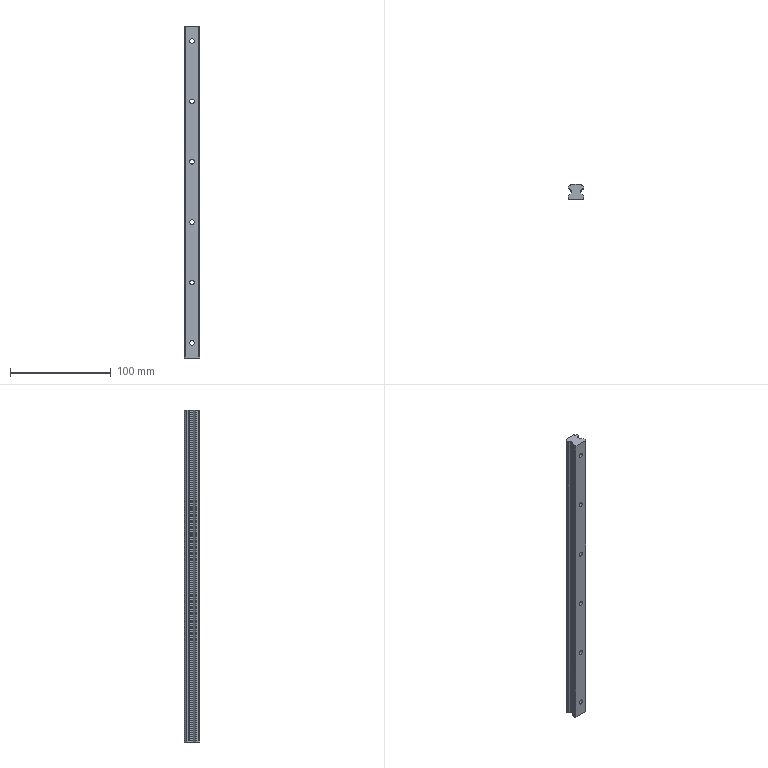Part | STEP file | 15 guide rail | 1 solid | 78 faces | box 15 x 15 x 330 mm | volume 60891 mm3 | plane 40 | cylinder 38 | commonest cylinder face diameters 4.5 x12 0.8 x8 6.5 x6 7.5 x6 3.24 x4 2 x2